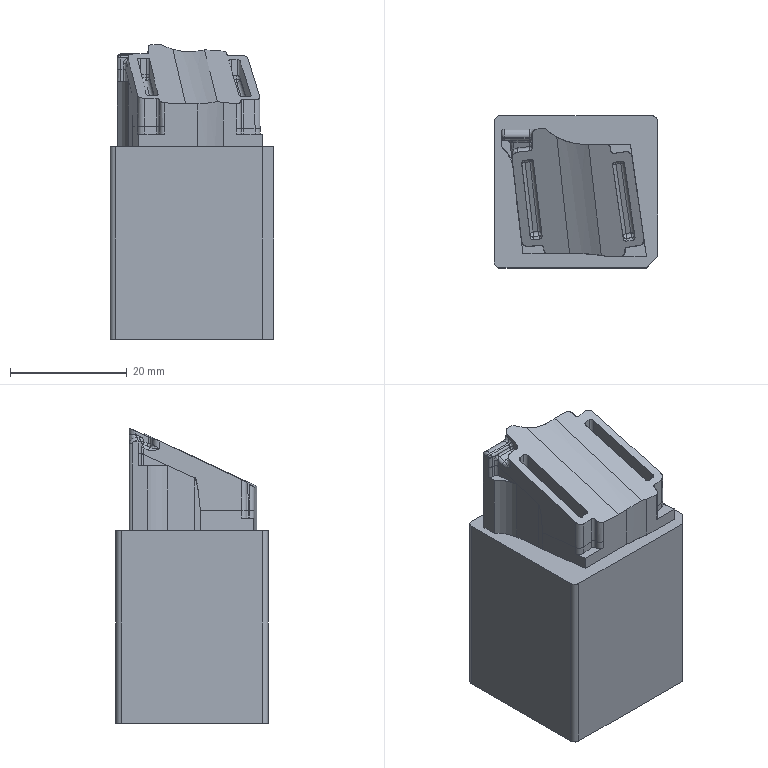NC program | NX | posted with a generic post | part box 28 x 26 x 50.455 mm
Lines 1 to 852 of 3612:
N10 G17 G21 G94 G90
(CONTOUR_AREA , TOOL : D6R3)
N12 T00 M6
N14 G54
N16 G17 G0 G90 X-10.629 Y6.566 S0 M3
N18 G43 Z10. H0
N20 Z1.729
N22 G94 G1 X-10.407 Y6.788 Z1.011 F250.
N24 X-10.061 Y7.134 Z0.4
N26 X-9.615 Y7.58 Z-0.064
N28 X-9.099 Y8.096 Z-0.349
N30 X-8.549 Y8.646 Z-0.436
N32 X-8.001 Y9.193 Z-0.318
N34 X-7.303 Y9.892 Z-0.032
N36 X-7.187 Y10.007 Z0.015
N38 X-6.981 Y10.073 Z0.034
N40 X-7.232 Y9.821 Z-0.069
N42 X-8.145 Y8.908 Z-0.443
N44 X-8.242 Y8.716 Z-0.526
N46 X-8.246 Y8.667 Z-0.549
N48 X-7.162 Y9.751 Z-0.105
N50 X-6.774 Y10.138 Z0.054
N52 X-6.681 Y10.168 Z0.062
N54 X-6.597 Y10.174 Z0.061
N56 X-7.091 Y9.68 Z-0.142
N58 X-8.256 Y8.515 Z-0.619
N60 X-8.267 Y8.363 Z-0.689
N62 X-7.02 Y9.609 Z-0.178
N64 X-6.444 Y10.186 Z0.058
N66 X-6.291 Y10.197 Z0.055
N68 X-6.95 Y9.539 Z-0.215
N70 X-8.223 Y8.266 Z-0.736
N72 X-8.278 Y8.211 Z-0.759
N74 X-8.289 Y8.059 Z-0.829
N76 X-8.152 Y8.195 Z-0.773
N78 X-6.879 Y9.468 Z-0.251
N80 X-6.146 Y10.201 Z0.049
N82 X-6.005 Z0.041
N84 X-6.808 Y9.398 Z-0.288
N86 X-8.081 Y8.125 Z-0.809
N88 X-8.299 Y7.907 Z-0.898
N90 X-8.31 Y7.755 Z-0.968
N92 X-8.011 Y8.054 Z-0.846
N94 X-7.235 Y8.83 Z-0.528
N96 X-6.738 Y9.327 Z-0.324
N98 X-5.864 Y10.201 Z0.034
N100 X-5.723 Z0.026
N102 X-6.515 Y9.408 Z-0.299
N104 X-7.324 Y8.6 Z-0.63
N106 X-7.94 Y7.983 Z-0.882
N108 X-8.32 Y7.604 Z-1.038
N110 X-8.329 Y7.453 Z-1.107
N112 X-7.869 Y7.913 Z-0.919
N114 X-7.352 Y8.43 Z-0.707
N116 X-6.328 Y9.454 Z-0.287
N118 X-5.581 Y10.201 Z0.018
N120 X-5.44 Z0.011
N122 X-6.189 Y9.452 Z-0.296
N124 X-7.341 Y8.3 Z-0.768
N126 X-7.799 Y7.842 Z-0.955
N128 X-8.339 Y7.302 Z-1.176
N130 X-8.348 Y7.152 Z-1.246
N132 X-7.728 Y7.772 Z-0.992
N134 X-7.35 Y8.149 Z-0.837
N136 X-6.044 Y9.456 Z-0.302
N138 X-5.299 Y10.201 Z0.003
N140 X-5.158 Z-0.004
N142 X-5.911 Y9.448 Z-0.313
N144 X-7.339 Y8.019 Z-0.898
N146 X-7.658 Y7.701 Z-1.028
N148 X-8.358 Y7.001 Z-1.315
N150 X-8.367 Y6.85 Z-1.384
N152 X-7.587 Y7.63 Z-1.065
N154 X-7.348 Y7.869 Z-0.967
N156 X-5.773 Y9.445 Z-0.322
N158 X-5.041 Y10.176 Z-0.022
N160 X-5.017 Y10.201 Z-0.012
N162 X-4.875 Z-0.02
N164 X-4.971 Y10.105 Z-0.059
N166 X-5.607 Y9.469 Z-0.319
N168 X-5.627 Y9.449 Z-0.327
N170 X-7.337 Y7.739 Z-1.028
N172 X-7.516 Y7.56 Z-1.101
N174 X-8.377 Y6.7 Z-1.454
N176 X-8.924 Y6.152 Z-1.571
N178 X-9.474 Y5.602 Z-1.485
N180 X-9.99 Y5.086 Z-1.2
N182 X-10.436 Y4.64 Z-0.735
N184 X-10.782 Y4.294 Z-0.124
N186 X-11.004 Y4.072 Z0.593
N188 Z1.943
N190 G0 Z4.343
N192 X-13.892 Y2.879
N194 Z0.196
N196 G1 X-13.67 Y3.101 Z-0.522
N198 X-13.324 Y3.447 Z-1.133
N200 X-12.878 Y3.893 Z-1.597
N202 X-12.362 Y4.409 Z-1.882
N204 X-11.811 Y4.96 Z-1.969
N206 X-11.264 Y5.507 Z-1.851
N208 X-11.034 Y5.737 Z-1.757
N210 X-10.651 Y6.015 Z-1.648
N212 X-10.581 Y6.049 Z-1.637
N214 X-10.839 Y5.791 Z-1.742
N216 X-11.457 Y5.173 Z-1.995
N218 X-11.535 Y4.954 Z-2.093
N220 X-10.768 Y5.72 Z-1.779
N222 X-10.35 Y6.139 Z-1.607
N224 X-10.14 Y6.208 Z-1.587
N226 X-10.697 Y5.65 Z-1.815
N228 X-11.612 Y4.736 Z-2.19
N230 X-11.689 Y4.517 Z-2.287
N232 X-10.627 Y5.579 Z-1.852
N234 X-9.93 Y6.276 Z-1.566
N236 X-9.72 Y6.345 Z-1.546
N238 X-10.556 Y5.509 Z-1.888
N240 X-11.683 Y4.382 Z-2.35
N242 X-11.669 Y4.254 Z-2.409
N244 X-10.486 Y5.438 Z-1.925
N246 X-9.522 Y6.401 Z-1.53
N248 X-9.332 Y6.45 Z-1.518
N250 X-10.415 Y5.367 Z-1.961
N252 X-11.655 Y4.127 Z-2.469
N254 X-11.641 Y4. Z-2.529
N256 X-11.617 Y4.024 Z-2.519
N258 X-10.616 Y5.025 Z-2.109
N260 X-10.327 Y5.314 Z-1.991
N262 X-9.142 Y6.499 Z-1.505
N264 X-8.952 Y6.548 Z-1.493
N266 X-9.001 Y6.499 Z-1.513
N268 X-10.061 Y5.439 Z-1.947
N270 X-10.731 Y4.769 Z-2.222
N272 X-11.547 Y3.953 Z-2.556
N274 X-11.627 Y3.873 Z-2.589
N276 X-11.613 Y3.745 Z-2.648
N278 X-11.476 Y3.883 Z-2.592
N280 X-10.76 Y4.599 Z-2.299
N282 X-9.885 Y5.474 Z-1.94
N284 X-8.93 Y6.428 Z-1.55
N286 X-8.762 Y6.597 Z-1.48
N288 X-8.571 Y6.646 Z-1.468
N290 X-8.86 Y6.358 Z-1.586
N292 X-9.715 Y5.502 Z-1.936
N294 X-10.769 Y4.448 Z-2.368
N296 X-11.405 Y3.812 Z-2.629
N298 X-11.599 Y3.618 Z-2.708
N300 X-11.585 Y3.491 Z-2.768
N302 X-11.335 Y3.741 Z-2.665
N304 X-10.758 Y4.318 Z-2.429
N306 X-9.565 Y5.511 Z-1.94
N308 X-8.789 Y6.287 Z-1.623
N310 X-8.381 Y6.695 Z-1.456
N312 X-7.874 Y7.202 Z-1.141
N314 X-7.442 Y7.634 Z-0.652
N316 X-7.113 Y7.963 Z-0.021
N318 X-6.912 Y8.164 Z0.708
N320 X-6.851 Y8.226 Z1.486
N322 X-6.934 Y8.142 Z2.261
N324 Z3.611
N326 G0 Z6.011
N328 X-11.215 Y0.117
N330 Z0.621
N332 G1 X-11.585 Y3.491 Z-2.773
N334 X-11.584 Y3.48
N336 X-11.57 Y3.365 Z-2.827
N338 X-11.264 Y3.671 Z-2.702
N340 X-10.747 Y4.188 Z-2.49
N342 X-9.395 Y5.54 Z-1.936
N344 X-8.718 Y6.216 Z-1.659
N346 X-7.446 Y7.489 Z-1.138
N348 X-7.346 Y7.589 Z-1.097
N350 X-5.497 Y9.438 Z-0.34
N352 X-4.9 Y10.035 Z-0.095
N354 X-4.735 Y10.2 Z-0.027
N356 X-4.649 Y10.144 Z-0.058
N358 X-4.829 Y9.964 Z-0.132
N360 X-5.347 Y9.447 Z-0.343
N362 X-7.355 Y7.438 Z-1.166
N364 X-7.375 Y7.418 Z-1.174
N366 X-8.648 Y6.146 Z-1.696
N368 X-9.244 Y5.549 Z-1.94
N370 X-10.736 Y4.058 Z-2.551
N372 X-11.193 Y3.6 Z-2.738
N374 X-11.554 Y3.24 Z-2.886
N376 X-11.538 Y3.114 Z-2.945
N378 X-11.123 Y3.53 Z-2.775
N380 X-10.725 Y3.927 Z-2.612
N382 X-9.074 Y5.578 Z-1.936
N384 X-8.577 Y6.075 Z-1.732
N386 X-7.344 Y7.308 Z-1.227
N388 X-5.196 Y9.456 Z-0.347
N390 X-4.759 Y9.893 Z-0.168
N392 X-4.564 Y10.088 Z-0.089
N394 X-4.479 Y10.032 Z-0.119
N396 X-4.688 Y9.823 Z-0.205
N398 X-5.066 Y9.445 Z-0.359
N400 X-7.353 Y7.158 Z-1.296
N402 X-8.507 Y6.004 Z-1.769
N404 X-8.924 Y5.587 Z-1.94
N406 X-10.694 Y3.817 Z-2.665
N408 X-11.052 Y3.459 Z-2.811
N410 X-11.523 Y2.988 Z-3.004
N412 X-11.507 Y2.863 Z-3.063
N414 X-10.982 Y3.388 Z-2.848
N416 X-10.683 Y3.687 Z-2.726
N418 X-8.754 Y5.616 Z-1.935
N420 X-8.436 Y5.934 Z-1.805
N422 X-7.342 Y7.028 Z-1.357
N424 X-4.995 Y9.374 Z-0.396
N426 X-4.618 Y9.752 Z-0.241
N428 X-4.394 Y9.976 Z-0.15
N430 X-4.309 Y9.919 Z-0.18
N432 X-4.547 Y9.682 Z-0.278
N434 X-4.925 Y9.304 Z-0.433
N436 X-7.351 Y6.877 Z-1.426
N438 X-8.365 Y5.863 Z-1.842
N440 X-8.604 Y5.625 Z-1.939
N442 X-10.672 Y3.556 Z-2.787
N444 X-10.911 Y3.318 Z-2.884
N446 X-11.491 Y2.737 Z-3.122
N448 X-11.476 Y2.612 Z-3.181
N450 X-10.84 Y3.247 Z-2.921
N452 X-10.661 Y3.426 Z-2.847
N454 X-8.434 Y5.653 Z-1.935
N456 X-8.295 Y5.793 Z-1.878
N458 X-7.34 Y6.747 Z-1.487
N460 X-4.854 Y9.233 Z-0.469
N462 X-4.476 Y9.611 Z-0.314
N464 X-4.224 Y9.863 Z-0.211
N466 X-4.139 Y9.807 Z-0.241
N468 X-4.406 Y9.54 Z-0.351
N470 X-4.784 Y9.162 Z-0.506
N472 X-7.349 Y6.597 Z-1.556
N474 X-8.224 Y5.722 Z-1.915
N476 X-8.284 Y5.662 Z-1.939
N478 X-10.65 Y3.296 Z-2.908
N480 X-10.77 Y3.176 Z-2.957
N482 X-11.46 Y2.486 Z-3.24
N484 X-11.445 Y2.359 Z-3.299
N486 X-10.699 Y3.106 Z-2.994
N488 X-10.62 Y3.185 Z-2.961
N490 X-8.134 Y5.671 Z-1.943
N492 X-7.338 Y6.467 Z-1.617
N494 X-4.693 Y9.112 Z-0.534
N496 X-4.335 Y9.47 Z-0.387
N498 X-4.054 Y9.751 Z-0.272
N500 X-3.969 Y9.695 Z-0.303
N502 X-4.265 Y9.399 Z-0.424
N504 X-4.622 Y9.041 Z-0.57
N506 X-7.347 Y6.317 Z-1.686
N508 X-7.964 Y5.7 Z-1.939
N510 X-10.609 Y3.055 Z-3.022
N512 X-10.628 Y3.035 Z-3.03
N514 X-11.43 Y2.233 Z-3.359
N516 X-11.415 Y2.107 Z-3.418
N518 X-10.608 Y2.914 Z-3.087
N520 X-7.794 Y5.729 Z-1.935
N522 X-7.336 Y6.186 Z-1.747
N524 X-4.552 Y8.971 Z-0.607
N526 X-4.194 Y9.328 Z-0.46
N528 X-3.884 Y9.639 Z-0.333
N530 X-3.799 Y9.582 Z-0.364
N532 X-4.123 Y9.258 Z-0.497
N534 X-4.441 Y8.94 Z-0.627
N536 X-4.461 Y8.92 Z-0.635
N538 X-10.595 Y2.787 Z-3.147
N540 X-11.4 Y1.981 Z-3.477
N542 X-11.385 Y1.855 Z-3.537
N544 X-10.574 Y2.666 Z-3.204
N546 X-4.391 Y8.849 Z-0.672
N548 X-4.371 Y8.869 Z-0.664
N550 X-4.053 Y9.187 Z-0.533
N552 X-3.714 Y9.526 Z-0.394
N554 X-3.628 Y9.47 Z-0.425
N556 X-3.982 Y9.117 Z-0.57
N558 X-4.3 Y8.798 Z-0.7
N560 X-4.32 Y8.779 Z-0.708
N562 X-10.558 Y2.54 Z-3.263
N564 X-11.37 Y1.728 Z-3.596
N566 X-11.355 Y1.602 Z-3.655
N568 X-10.548 Y2.41 Z-3.324
N570 X-9.082 Y3.875 Z-2.724
N572 X-9.003 Y3.955 Z-2.692
N574 X-8.903 Y4.054 Z-2.651
N576 X-4.23 Y8.728 Z-0.737
N578 X-3.911 Y9.046 Z-0.606
N580 X-3.543 Y9.415 Z-0.455
N582 X-3.457 Y9.359 Z-0.486
N584 X-3.841 Y8.975 Z-0.643
N586 X-4.139 Y8.677 Z-0.765
N588 X-8.693 Y4.123 Z-2.63
N590 X-8.932 Y3.884 Z-2.728
N592 X-9.171 Y3.646 Z-2.826
N594 X-10.526 Y2.29 Z-3.381
N596 X-11.34 Y1.476 Z-3.714
N598 X-11.325 Y1.35 Z-3.774
N600 X-10.507 Y2.168 Z-3.439
N602 X-9.16 Y3.515 Z-2.887
N604 X-8.861 Y3.814 Z-2.765
N606 X-8.523 Y4.152 Z-2.626
N608 X-4.068 Y8.606 Z-0.802
N610 X-3.77 Y8.905 Z-0.679
N612 X-3.372 Y9.303 Z-0.516
N614 X-3.287 Y9.247 Z-0.546
N616 X-3.7 Y8.834 Z-0.716
N618 X-3.978 Y8.556 Z-0.83
N620 X-8.373 Y4.161 Z-2.63
N622 X-8.791 Y3.743 Z-2.801
N624 X-9.149 Y3.385 Z-2.948
N626 X-10.492 Y2.042 Z-3.498
N628 X-11.309 Y1.225 Z-3.833
N630 X-11.293 Y1.099 Z-3.891
N632 X-11.266 Y1.127 Z-3.88
N634 X-10.48 Y1.913 Z-3.558
N636 X-9.138 Y3.255 Z-3.009
N638 X-8.72 Y3.672 Z-2.838
N640 X-8.203 Y4.189 Z-2.626
N642 X-3.887 Y8.505 Z-0.858
N644 X-3.629 Y8.764 Z-0.752
N646 X-3.201 Y9.191 Z-0.577
N648 X-3.116 Y9.135 Z-0.607
N650 X-3.558 Y8.693 Z-0.788
N652 X-3.817 Y8.434 Z-0.895
N654 X-8.053 Y4.198 Z-2.63
N656 X-8.649 Y3.602 Z-2.874
N658 X-9.107 Y3.144 Z-3.062
N660 X-10.459 Y1.792 Z-3.615
N662 X-11.195 Y1.056 Z-3.917
N664 X-11.277 Y0.974 Z-3.95
N666 X-11.261 Y0.849 Z-4.009
N668 X-11.124 Y0.986 Z-3.953
N670 X-10.448 Y1.662 Z-3.676
N672 X-9.096 Y3.014 Z-3.122
N674 X-8.579 Y3.531 Z-2.911
N676 X-7.883 Y4.227 Z-2.626
N678 X-3.726 Y8.384 Z-0.923
N680 X-3.488 Y8.622 Z-0.825
N682 X-3.031 Y9.079 Z-0.637
N684 X-2.945 Y9.023 Z-0.666
N686 X-3.417 Y8.552 Z-0.861
N688 X-3.636 Y8.333 Z-0.952
N690 X-7.733 Y4.236 Z-2.63
N692 X-8.508 Y3.46 Z-2.947
N694 X-9.085 Y2.884 Z-3.183
N696 X-10.437 Y1.531 Z-3.737
N698 X-11.054 Y0.915 Z-3.99
N700 X-11.246 Y0.723 Z-4.068
N702 X-11.23 Y0.598 Z-4.127
N704 X-10.983 Y0.844 Z-4.026
N706 X-10.426 Y1.401 Z-3.798
N708 X-9.074 Y2.753 Z-3.244
N710 X-8.438 Y3.39 Z-2.984
N712 X-7.582 Y4.245 Z-2.633
N714 X-3.545 Y8.282 Z-0.98
N716 X-3.346 Y8.481 Z-0.898
N718 X-2.86 Y8.968 Z-0.695
N720 X-2.775 Y8.911 Z-0.724
N722 X-3.276 Y8.41 Z-0.934
N724 X-3.435 Y8.251 Z-1.
N726 X-3.455 Y8.231 Z-1.008
N728 X-7.452 Y4.234 Z-2.646
N730 X-8.367 Y3.319 Z-3.02
N732 X-9.063 Y2.623 Z-3.305
N734 X-10.415 Y1.271 Z-3.859
N736 X-10.913 Y0.774 Z-4.063
N738 X-11.214 Y0.472 Z-4.186
N740 X-11.198 Y0.347 Z-4.245
N742 X-10.842 Y0.703 Z-4.099
N744 X-10.385 Y1.16 Z-3.912
N746 X-9.052 Y2.493 Z-3.366
N748 X-8.296 Y3.249 Z-3.057
N750 X-7.362 Y4.183 Z-2.674
N752 X-3.364 Y8.181 Z-1.037
N754 X-3.205 Y8.34 Z-0.97
N756 X-2.69 Y8.854 Z-0.752
N758 X-2.606 Y8.798 Z-0.775
N760 X-3.135 Y8.269 Z-1.007
N762 X-3.274 Y8.13 Z-1.065
N764 X-7.271 Y4.133 Z-2.702
N766 X-8.226 Y3.178 Z-3.093
N768 X-9.021 Y2.382 Z-3.419
N770 X-10.374 Y1.03 Z-3.973
N772 X-10.771 Y0.632 Z-4.136
N774 X-11.182 Y0.221 Z-4.304
N776 X-11.167 Y0.096 Z-4.363
N778 X-10.701 Y0.562 Z-4.172
N780 X-10.363 Y0.9 Z-4.034
N782 X-9.01 Y2.252 Z-3.48
N784 X-8.155 Y3.107 Z-3.13
N786 X-7.22 Y4.042 Z-2.747
N788 X-3.203 Y8.059 Z-1.102
N790 X-3.064 Y8.199 Z-1.044
N792 X-2.521 Y8.741 Z-0.802
N794 X-2.436 Y8.685 Z-0.829
N796 X-2.993 Y8.128 Z-1.079
N798 X-3.133 Y7.989 Z-1.138
N800 X-7.15 Y3.971 Z-2.784
N802 X-8.084 Y3.037 Z-3.166
N804 X-8.999 Y2.122 Z-3.541
N806 X-10.352 Y0.77 Z-4.095
N808 X-10.63 Y0.491 Z-4.209
N810 X-11.152 Y-0.031 Z-4.423
N812 X-11.137 Y-0.157 Z-4.482
N814 X-10.559 Y0.421 Z-4.245
N816 X-10.341 Y0.639 Z-4.156
N818 X-8.988 Y1.992 Z-3.602
N820 X-8.014 Y2.966 Z-3.203
N822 X-7.119 Y3.861 Z-2.836
N824 X-3.122 Y7.858 Z-1.199
N826 X-2.923 Y8.057 Z-1.115
N828 X-2.352 Y8.628 Z-0.856
N830 X-2.267 Y8.572 Z-0.882
N832 X-2.852 Y7.987 Z-1.15
N834 X-3.111 Y7.728 Z-1.26
N836 X-7.108 Y3.731 Z-2.897
N838 X-7.943 Y2.896 Z-3.239
N840 X-8.977 Y1.861 Z-3.663
N842 X-10.33 Y0.509 Z-4.217
N844 X-10.489 Y0.35 Z-4.282
N846 X-11.122 Y-0.283 Z-4.541
N848 X-11.107 Y-0.41 Z-4.601
N850 X-10.418 Y0.279 Z-4.318
N852 X-10.299 Y0.399 Z-4.27
N854 X-8.947 Y1.751 Z-3.716
N856 X-7.873 Y2.825 Z-3.276
N858 X-7.077 Y3.62 Z-2.95
N860 X-3.1 Y7.598 Z-1.321
N862 X-2.781 Y7.916 Z-1.186
N864 X-2.178 Y8.52 Z-0.906
N866 X-2.085 Y8.471 Z-0.927
N868 X-2.711 Y7.845 Z-1.221
N870 X-3.089 Y7.468 Z-1.382
N872 X-7.066 Y3.49 Z-3.011
N874 X-7.802 Y2.754 Z-3.312
N876 X-8.936 Y1.621 Z-3.777
N878 X-10.288 Y0.268 Z-4.331
N880 X-10.348 Y0.209 Z-4.355
N882 X-11.092 Y-0.536 Z-4.66
N884 X-11.077 Y-0.662 Z-4.719
N886 X-10.277 Y0.138 Z-4.392
N888 X-8.925 Y1.49 Z-3.838
N890 X-7.731 Y2.684 Z-3.349
N892 X-7.055 Y3.36 Z-3.072
N894 X-3.078 Y7.337 Z-1.443
N896 X-2.64 Y7.775 Z-1.255
N898 X-1.992 Y8.423 Z-0.948
N900 X-1.893 Y8.38 Z-0.963
N902 X-2.57 Y7.704 Z-1.289
N904 X-3.057 Y7.217 Z-1.5
N906 X-7.044 Y3.23 Z-3.133
N908 X-7.661 Y2.613 Z-3.385
N910 X-8.914 Y1.36 Z-3.899
N912 X-10.269 Y0.005 Z-4.454
N914 X-11.062 Y-0.789 Z-4.779
N916 X-11.047 Y-0.914 Z-4.838
N918 X-10.256 Y-0.124 Z-4.514
N920 X-8.903 Y1.23 Z-3.96
N922 X-8.863 Y1.27 Z-3.943
N924 X-7.59 Y2.542 Z-3.422
N926 X-7.033 Y3.099 Z-3.194
N928 X-3.043 Y7.089 Z-1.56
N930 X-2.499 Y7.634 Z-1.324
N932 X-1.841 Y8.292 Z-1.006
N934 X-1.795 Y8.338 Z-0.979
N936 X-1.697 Y8.295 Z-0.995
N938 X-1.742 Y8.249 Z-1.022
N940 X-2.085 Y7.906 Z-1.194
N942 X-2.257 Y7.734 Z-1.278
N944 X-2.428 Y7.563 Z-1.358
N946 X-3.025 Y6.966 Z-1.618
N948 X-7.002 Y2.989 Z-3.247
N950 X-7.52 Y2.472 Z-3.458
N952 X-8.792 Y1.199 Z-3.98
N954 X-8.872 Y1.119 Z-4.012
N956 X-10.236 Y-0.245 Z-4.571
N958 X-11.031 Y-1.04 Z-4.897
N960 X-11.015 Y-1.165 Z-4.956
N962 X-10.221 Y-0.371 Z-4.63
N964 X-8.861 Y0.989 Z-4.073
N966 X-8.722 Y1.128 Z-4.016
N968 X-7.449 Y2.401 Z-3.495
N970 X-6.991 Y2.859 Z-3.308
N972 X-3.014 Y6.836 Z-1.679
N974 X-2.994 Y6.856 Z-1.67
N976 X-2.358 Y7.492 Z-1.392
N978 X-2.001 Y7.849 Z-1.219
N980 X-1.644 Y8.206 Z-1.039
N982 X-1.598 Y8.252 Z-1.01
N984 X-1.5 Y8.209 Z-1.026
N986 X-1.545 Y8.163 Z-1.055
N988 X-1.916 Y7.792 Z-1.245
N990 X-2.102 Y7.607 Z-1.337
N992 X-2.287 Y7.422 Z-1.426
N994 X-3.003 Y6.706 Z-1.74
N996 X-6.981 Y2.728 Z-3.369
N998 X-7.378 Y2.331 Z-3.532
N1000 X-8.651 Y1.058 Z-4.053
N1002 X-8.85 Y0.859 Z-4.134
N1004 X-10.211 Y-0.502 Z-4.692
N1006 X-10.999 Y-1.291 Z-5.015
N1008 X-10.984 Y-1.416 Z-5.074
N1010 X-10.19 Y-0.622 Z-4.748
N1012 X-8.839 Y0.729 Z-4.195
N1014 X-8.58 Y0.987 Z-4.089
N1016 X-7.308 Y2.26 Z-3.568
N1018 X-6.97 Y2.598 Z-3.43
N1020 X-2.992 Y6.575 Z-1.8
N1022 X-2.216 Y7.351 Z-1.459
N1024 X-1.832 Y7.736 Z-1.27
N1026 X-1.447 Y8.12 Z-1.07
N1028 X-1.402 Y8.166 Z-1.042
N1030 X-1.303 Y8.123 Z-1.057
N1032 X-1.947 Y7.48 Z-1.395
N1034 X-2.146 Y7.28 Z-1.492
N1036 X-2.961 Y6.465 Z-1.853
N1038 X-2.981 Y6.445 Z-1.861
N1040 X-6.959 Y2.468 Z-3.491
N1042 X-7.237 Y2.189 Z-3.605
N1044 X-8.51 Y0.916 Z-4.126
N1046 X-8.828 Y0.598 Z-4.256
N1048 X-10.172 Y-0.745 Z-4.806
N1050 X-10.968 Y-1.542 Z-5.133
N1052 X-10.953 Y-1.668 Z-5.192
N1054 X-10.157 Y-0.872 Z-4.866
N1056 X-8.817 Y0.468 Z-4.317
N1058 X-8.439 Y0.846 Z-4.162
N1060 X-7.166 Y2.119 Z-3.641
N1062 X-6.948 Y2.337 Z-3.551
N1064 X-2.97 Y6.315 Z-1.922
N1066 X-2.712 Y6.573 Z-1.813
N1068 X-2.075 Y7.21 Z-1.524
N1070 X-1.663 Y7.622 Z-1.317
N1072 X-1.205 Y8.08 Z-1.073
N1074 X-1.163 Y8.062 Z-1.08
N1076 X-1.1 Y8.044 Z-1.082
N1078 X-1.577 Y7.567 Z-1.34
N1080 X-1.791 Y7.353 Z-1.449
N1082 X-2.005 Y7.139 Z-1.556
N1084 X-2.641 Y6.503 Z-1.848
N1086 X-2.8 Y6.344 Z-1.917
N1088 X-2.939 Y6.205 Z-1.975
N1090 X-6.917 Y2.227 Z-3.604
N1092 X-7.096 Y2.048 Z-3.678
N1094 X-8.369 Y0.775 Z-4.199
N1096 X-8.786 Y0.358 Z-4.37
N1098 X-10.146 Y-1.002 Z-4.927
N1100 X-10.914 Y-1.77 Z-5.241
N1102 X-10.938 Y-1.794 Z-5.251
N1104 X-10.923 Y-1.92 Z-5.311
N1106 X-10.844 Y-1.841 Z-5.278
N1108 X-10.128 Y-1.125 Z-4.985
N1110 X-8.775 Y0.227 Z-4.431
N1112 X-8.298 Y0.705 Z-4.235
N1114 X-7.025 Y1.977 Z-3.714
N1116 X-6.906 Y2.097 Z-3.665
N1118 X-2.928 Y6.074 Z-2.036
N1120 X-2.57 Y6.432 Z-1.883
N1122 X-1.934 Y7.069 Z-1.588
N1124 X-1.486 Y7.516 Z-1.361
N1126 X-0.99 Y8.012 Z-1.086
N1128 X-0.881 Y7.981 Z-1.091
N1130 X-0.929 Y7.932 Z-1.122
N1132 X-1.396 Y7.465 Z-1.381
N1134 X-1.63 Y7.231 Z-1.502
N1136 X-1.863 Y6.998 Z-1.62
N1138 X-2.5 Y6.362 Z-1.918
N1140 X-2.917 Y5.944 Z-2.097
N1142 X-6.895 Y1.966 Z-3.726
N1144 X-6.955 Y1.907 Z-3.751
N1146 X-8.227 Y0.634 Z-4.272
N1148 X-8.764 Y0.097 Z-4.492
N1150 X-10.117 Y-1.255 Z-5.046
N1152 X-10.773 Y-1.912 Z-5.315
N1154 X-10.908 Y-2.047 Z-5.37
N1156 X-10.893 Y-2.173 Z-5.429
N1158 X-10.702 Y-1.982 Z-5.351
N1160 X-10.106 Y-1.386 Z-5.107
N1162 X-8.753 Y-0.033 Z-4.553
N1164 X-8.157 Y0.563 Z-4.308
N1166 X-6.884 Y1.836 Z-3.787
N1168 X-2.906 Y5.814 Z-2.158
N1170 X-2.429 Y6.291 Z-1.951
N1172 X-1.793 Y6.927 Z-1.652
N1174 X-1.306 Y7.414 Z-1.4
N1176 X-0.82 Y7.9 Z-1.127
N1178 X-0.771 Y7.949 Z-1.095
N1180 X-0.662 Y7.917 Z-1.099
N1182 X-0.71 Y7.869 Z-1.133
N1184 X-1.216 Y7.363 Z-1.418
N1186 X-1.469 Y7.11 Z-1.555
N1188 X-1.722 Y6.857 Z-1.685
N1190 X-2.359 Y6.22 Z-1.985
N1192 X-2.895 Y5.683 Z-2.219
N1194 X-6.873 Y1.706 Z-3.848
N1196 X-8.086 Y0.493 Z-4.345
N1198 X-8.742 Y-0.164 Z-4.614
N1200 X-10.095 Y-1.516 Z-5.168
N1202 X-10.632 Y-2.053 Z-5.388
N1204 X-10.878 Y-2.3 Z-5.489
N1206 X-10.864 Y-2.426 Z-5.548
N1208 X-10.561 Y-2.123 Z-5.424
N1210 X-10.064 Y-1.626 Z-5.22
N1212 X-8.712 Y-0.274 Z-4.667
N1214 X-8.015 Y0.422 Z-4.381
N1216 X-6.842 Y1.595 Z-3.901
N1218 X-2.885 Y5.553 Z-2.28
N1220 X-2.288 Y6.15 Z-2.019
N1222 X-1.651 Y6.786 Z-1.716
N1224 X-1.389 Y7.049 Z-1.581
N1226 X-1.126 Y7.312 Z-1.437
N1228 X-0.6 Y7.837 Z-1.135
N1230 X-0.552 Y7.886 Z-1.103
N1232 X-0.442 Y7.854 Z-1.107
N1234 X-1.036 Y7.261 Z-1.456
N1236 X-1.308 Y6.988 Z-1.605
N1238 X-1.581 Y6.715 Z-1.746
N1240 X-2.217 Y6.079 Z-2.052
N1242 X-2.834 Y5.463 Z-2.325
N1244 X-2.854 Y5.443 Z-2.333
N1246 X-6.831 Y1.465 Z-3.962
N1248 X-7.945 Y0.352 Z-4.418
N1250 X-8.701 Y-0.404 Z-4.728
N1252 X-10.053 Y-1.757 Z-5.281
N1254 X-10.49 Y-2.194 Z-5.461
N1256 X-10.848 Y-2.552 Z-5.607
N1258 X-10.832 Y-2.677 Z-5.666
N1260 X-10.42 Y-2.265 Z-5.497
N1262 X-10.042 Y-1.887 Z-5.342
N1264 X-8.69 Y-0.534 Z-4.788
N1266 X-7.874 Y0.281 Z-4.454
N1268 X-6.82 Y1.335 Z-4.023
N1270 X-2.843 Y5.312 Z-2.394
N1272 X-2.823 Y5.332 Z-2.386
N1274 X-2.783 Y5.372 Z-2.369
N1276 X-1.51 Y6.645 Z-1.777
N1278 X-0.946 Y7.209 Z-1.473
N1280 X-0.333 Y7.823 Z-1.112
N1282 X-0.214 Y7.8 Z-1.106
N1284 X-0.853 Y7.161 Z-1.488
N1286 X-1.146 Y6.868 Z-1.651
N1288 X-1.44 Y6.574 Z-1.808
N1290 X-2.712 Y5.301 Z-2.405
N1292 X-2.832 Y5.182 Z-2.455
N1294 X-6.809 Y1.205 Z-4.084
N1296 X-7.804 Y0.21 Z-4.491
N1298 X-8.679 Y-0.665 Z-4.849
N1300 X-10.031 Y-2.017 Z-5.403
N1302 X-10.349 Y-2.335 Z-5.534
N1304 X-10.816 Y-2.803 Z-5.725
N1306 X-10.801 Y-2.928 Z-5.784
N1308 X-10.279 Y-2.406 Z-5.57
N1310 X-10.02 Y-2.147 Z-5.464
N1312 X-8.668 Y-0.795 Z-4.91
N1314 X-7.733 Y0.14 Z-4.528
N1316 X-6.798 Y1.074 Z-4.145
N1318 X-2.821 Y5.052 Z-2.516
N1320 X-2.801 Y5.072 Z-2.507
N1322 X-2.642 Y5.231 Z-2.44
N1324 X-1.369 Y6.504 Z-1.838
N1326 X-0.757 Y7.116 Z-1.501
N1328 X-0.093 Y7.779 Z-1.096
N1330 X0.027 Y7.759 Z-1.087
N1332 X-0.026 Y7.706 Z-1.126
N1334 X-1.298 Y6.433 Z-1.867
N1336 X-2.571 Y5.16 Z-2.475
N1338 X-2.81 Y4.922 Z-2.577
N1340 X-6.787 Y0.944 Z-4.206
N1342 X-7.662 Y0.069 Z-4.564
N1344 X-8.637 Y-0.905 Z-4.963
N1346 X-9.989 Y-2.258 Z-5.517
N1348 X-10.208 Y-2.477 Z-5.607
N1350 X-10.785 Y-3.054 Z-5.843
N1352 X-10.769 Y-3.179 Z-5.902
N1354 X-10.137 Y-2.547 Z-5.643
N1356 X-9.978 Y-2.388 Z-5.578
N1358 X-8.626 Y-1.036 Z-5.024
N1360 X-7.592 Y-0.002 Z-4.601
N1362 X-6.756 Y0.834 Z-4.258
N1364 X-2.799 Y4.791 Z-2.638
N1366 X-2.501 Y5.09 Z-2.51
N1368 X-1.228 Y6.362 Z-1.896
N1370 X0.045 Y7.635 Z-1.15
N1372 X0.148 Y7.738 Z-1.079
N1374 X0.269 Y7.717 Z-1.07
N1376 X0.116 Y7.565 Z-1.174
N1378 X-1.157 Y6.292 Z-1.925
N1380 X-2.43 Y5.019 Z-2.545
N1382 X-2.788 Y4.661 Z-2.699
N1384 X-6.745 Y0.703 Z-4.319
N1386 X-7.521 Y-0.072 Z-4.637
N1388 X-8.615 Y-1.166 Z-5.085
N1390 X-9.967 Y-2.518 Z-5.639
N1392 X-10.067 Y-2.618 Z-5.68
N1394 X-10.754 Y-3.305 Z-5.961
N1396 X-10.739 Y-3.431 Z-6.02
N1398 X-9.996 Y-2.688 Z-5.716
N1400 X-9.956 Y-2.649 Z-5.7
N1402 X-8.604 Y-1.296 Z-5.146
N1404 X-7.45 Y-0.143 Z-4.674
N1406 X-6.735 Y0.573 Z-4.38
N1408 X-2.757 Y4.551 Z-2.751
N1410 X-2.359 Y4.948 Z-2.578
N1412 X-1.087 Y6.221 Z-1.954
N1414 X0.186 Y7.494 Z-1.197
N1416 X0.389 Y7.697 Z-1.063
N1418 X0.51 Y7.676 Z-1.053
N1420 X0.257 Y7.423 Z-1.219
N1422 X-1.016 Y6.151 Z-1.983
N1424 X-2.289 Y4.878 Z-2.612
N1426 X-2.746 Y4.42 Z-2.812
N1428 X-6.724 Y0.443 Z-4.441
N1430 X-7.38 Y-0.213 Z-4.71
N1432 X-8.593 Y-1.427 Z-5.207
N1434 X-9.949 Y-2.782 Z-5.762
N1436 X-10.724 Y-3.558 Z-6.08
N1438 X-10.709 Y-3.684 Z-6.139
N1440 X-9.93 Y-2.905 Z-5.82
N1442 X-8.582 Y-1.557 Z-5.268
N1444 X-7.309 Y-0.284 Z-4.747
N1446 X-6.713 Y0.313 Z-4.502
N1448 X-2.735 Y4.29 Z-2.873
N1450 X-2.218 Y4.807 Z-2.646
N1452 X-0.945 Y6.08 Z-2.011
N1454 X0.328 Y7.353 Z-1.242
N1456 X0.64 Y7.665 Z-1.035
N1458 X0.772 Y7.656 Z-1.019
N1460 X0.398 Y7.282 Z-1.265
N1462 X-0.875 Y6.009 Z-2.038
N1464 X-2.147 Y4.736 Z-2.678
N1466 X-2.466 Y4.418 Z-2.824
N1468 X-2.625 Y4.259 Z-2.893
N1470 X-2.704 Y4.18 Z-2.926
N1472 X-2.724 Y4.16 Z-2.934
N1474 X-6.682 Y0.202 Z-4.555
N1476 X-7.239 Y-0.355 Z-4.783
N1478 X-8.511 Y-1.627 Z-5.304
N1480 X-8.551 Y-1.667 Z-5.321
N1482 X-9.918 Y-3.034 Z-5.881
N1484 X-10.694 Y-3.81 Z-6.198
N1486 X-10.679 Y-3.937 Z-6.258
N1488 X-9.899 Y-3.156 Z-5.938
N1490 X-8.54 Y-1.798 Z-5.382
N1492 X-8.441 Y-1.698 Z-5.341
N1494 X-7.168 Y-0.425 Z-4.82
N1496 X-6.671 Y0.072 Z-4.616
N1498 X-2.713 Y4.029 Z-2.995
N1500 X-2.395 Y4.348 Z-2.858
N1502 X-2.077 Y4.666 Z-2.71
N1504 X-0.804 Y5.939 Z-2.065
N1506 X0.469 Y7.211 Z-1.288
N1508 X0.847 Y7.59 Z-1.032
N1510 X0.904 Y7.646 Z-1.002
N1512 X1.036 Y7.637 Z-0.984
N1514 X0.979 Y7.581 Z-1.012
N1516 X0.539 Y7.141 Z-1.311
N1518 X-0.733 Y5.868 Z-2.093
N1520 X-2.006 Y4.595 Z-2.742
N1522 X-2.702 Y3.899 Z-3.056
N1524 X-6.66 Y-0.058 Z-4.677
N1526 X-7.097 Y-0.496 Z-4.856
N1528 X-8.37 Y-1.769 Z-5.377
N1530 X-8.529 Y-1.928 Z-5.443
N1532 X-9.885 Y-3.283 Z-5.998
N1534 X-10.665 Y-4.063 Z-6.317
N1536 X-10.649 Y-4.189 Z-6.376
N1538 X-9.86 Y-3.4 Z-6.053
N1540 X-8.518 Y-2.058 Z-5.504
N1542 X-8.3 Y-1.839 Z-5.414
N1544 X-7.027 Y-0.567 Z-4.893
N1546 X-6.649 Y-0.189 Z-4.738
N1548 X-2.691 Y3.769 Z-3.117
N1550 X-2.572 Y3.888 Z-3.067
N1552 X-1.936 Y4.525 Z-2.774
N1554 X-0.663 Y5.797 Z-2.12
N1556 X0.61 Y7.07 Z-1.333
N1558 X1.111 Y7.572 Z-0.995
N1560 X1.168 Y7.628 Z-0.967
N1562 X1.3 Y7.619 Z-0.947
N1564 X0.681 Y7. Z-1.356
N1566 X-0.592 Y5.727 Z-2.148
N1568 X-1.865 Y4.454 Z-2.807
N1570 X-2.621 Y3.698 Z-3.153
N1572 X-2.641 Y3.678 Z-3.162
N1574 X-2.66 Y3.658 Z-3.17
N1576 X-6.638 Y-0.319 Z-4.799
N1578 X-6.956 Y-0.637 Z-4.929
N1580 X-8.229 Y-1.91 Z-5.451
N1582 X-8.507 Y-2.188 Z-5.565
N1584 X-9.855 Y-3.537 Z-6.117
N1586 X-10.634 Y-4.315 Z-6.435
N1588 X-10.618 Y-4.44 Z-6.494
N1590 X-9.838 Y-3.661 Z-6.175
N1592 X-8.476 Y-2.299 Z-5.617
N1594 X-8.158 Y-1.981 Z-5.487
N1596 X-6.886 Y-0.708 Z-4.966
N1598 X-6.607 Y-0.429 Z-4.852
N1600 X-2.649 Y3.528 Z-3.231
N1602 X-2.431 Y3.747 Z-3.137
N1604 X-1.794 Y4.383 Z-2.841
N1606 X-0.522 Y5.656 Z-2.177
N1608 X0.751 Y6.929 Z-1.378
N1610 X1.434 Y7.612 Z-0.932
N1612 X1.573 Y7.61 Z-0.915
N1614 X0.822 Y6.858 Z-1.398
N1616 X-0.451 Y5.586 Z-2.207
N1618 X-1.724 Y4.313 Z-2.875
N1620 X-2.36 Y3.676 Z-3.172
N1622 X-2.519 Y3.517 Z-3.241
N1624 X-2.639 Y3.398 Z-3.292
N1626 X-6.596 Y-0.56 Z-4.913
N1628 X-6.815 Y-0.778 Z-5.002
N1630 X-8.088 Y-2.051 Z-5.524
N1632 X-8.466 Y-2.429 Z-5.678
N1634 X-9.824 Y-3.788 Z-6.235
N1636 X-10.602 Y-4.566 Z-6.553
N1638 X-10.586 Y-4.691 Z-6.612
N1640 X-10.563 Y-4.667 Z-6.603
N1642 X-9.814 Y-3.919 Z-6.296
N1644 X-8.455 Y-2.559 Z-5.739
N1646 X-8.017 Y-2.122 Z-5.56
N1648 X-6.744 Y-0.849 Z-5.039
N1650 X-6.585 Y-0.69 Z-4.974
N1652 X-2.628 Y3.268 Z-3.353
N1654 X-2.608 Y3.288 Z-3.345
N1656 X-2.289 Y3.606 Z-3.205
N1658 X-1.653 Y4.242 Z-2.909
N1660 X-0.38 Y5.515 Z-2.233
N1662 X0.892 Y6.788 Z-1.419
N1664 X1.083 Y6.978 Z-1.289
N1666 X1.713 Y7.608 Z-0.897
N1668 X1.852 Y7.606 Z-0.909
N1670 X1.792 Y7.546 Z-0.917
N1672 X1.378 Y7.132 Z-1.169
N1674 X1.17 Y6.924 Z-1.296
N1676 X0.963 Y6.717 Z-1.44
N1678 X-0.31 Y5.444 Z-2.259
N1680 X-1.582 Y4.171 Z-2.944
N1682 X-2.219 Y3.535 Z-3.239
N1684 X-2.617 Y3.137 Z-3.414
N1686 X-6.574 Y-0.82 Z-5.035
N1688 X-6.674 Y-0.92 Z-5.075
N1690 X-7.946 Y-2.192 Z-5.597
N1692 X-8.444 Y-2.69 Z-5.8
N1694 X-9.796 Y-4.042 Z-6.354
N1696 X-10.492 Y-4.738 Z-6.639
N1698 X-10.571 Y-4.817 Z-6.671
N1700 X-10.555 Y-4.942 Z-6.73
N1702 X-10.421 Y-4.809 Z-6.676